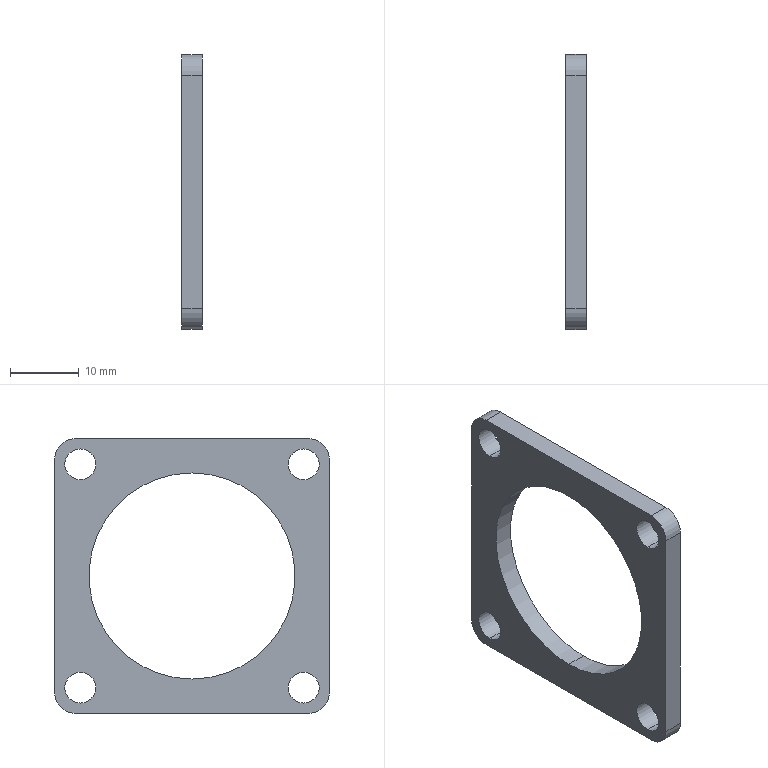Part | SolidWorks | features BaseBody 1 | 1 solid | 20 faces | box 3 x 40 x 40 mm | volume 2465 mm3 | cylinder 14 | plane 6 | commonest cylinder face diameters 4.5 x8 6 x4 30 x2
STEP:
#1=CARTESIAN_POINT('',(298.479,1907.044,-147.5));
#2=VERTEX_POINT('',#1);
#3=CARTESIAN_POINT('',(298.479,1907.044,-177.5));
#4=VERTEX_POINT('',#3);
#5=CARTESIAN_POINT('',(298.479,1907.044,-162.5));
#6=DIRECTION('',(1.,0.,0.));
#7=DIRECTION('',(0.,0.,-1.));
#8=AXIS2_PLACEMENT_3D('',#5,#6,#7);
#9=CIRCLE('',#8,15.);
#10=EDGE_CURVE('',#2,#4,#9,.T.);
#11=ORIENTED_EDGE('',*,*,#10,.F.);
#12=CARTESIAN_POINT('',(301.479,1907.044,-147.5));
#13=VERTEX_POINT('',#12);
#14=CARTESIAN_POINT('',(244.831,1907.044,-147.5));
#15=DIRECTION('',(1.,0.,0.));
#16=VECTOR('',#15,1000.);
#17=LINE('',#14,#16);
#18=EDGE_CURVE('',#2,#13,#17,.T.);
#19=ORIENTED_EDGE('',*,*,#18,.T.);
#20=CARTESIAN_POINT('',(301.479,1907.044,-177.5));
#21=VERTEX_POINT('',#20);
#22=CARTESIAN_POINT('',(301.479,1907.044,-162.5));
#23=DIRECTION('',(-1.,0.,0.));
#24=DIRECTION('',(0.,0.,-1.));
#25=AXIS2_PLACEMENT_3D('',#22,#23,#24);
#26=CIRCLE('',#25,15.);
#27=EDGE_CURVE('',#21,#13,#26,.T.);
#28=ORIENTED_EDGE('',*,*,#27,.F.);
#29=CARTESIAN_POINT('',(244.831,1907.044,-177.5));
#30=DIRECTION('',(1.,0.,0.));
#31=VECTOR('',#30,1000.);
#32=LINE('',#29,#31);
#33=EDGE_CURVE('',#4,#21,#32,.T.);
#34=ORIENTED_EDGE('',*,*,#33,.F.);
#35=EDGE_LOOP('',(#11,#19,#28,#34));
#36=FACE_OUTER_BOUND('',#35,.T.);
#37=CARTESIAN_POINT('',(244.831,1907.044,-162.5));
#38=DIRECTION('',(1.,0.,0.));
#39=DIRECTION('',(0.,0.,-1.));
#40=AXIS2_PLACEMENT_3D('',#37,#38,#39);
#41=CYLINDRICAL_SURFACE('',#40,15.);
#42=ADVANCED_FACE('',(#36),#41,.F.);
#43=CARTESIAN_POINT('',(298.479,1890.781,-176.513));
#44=VERTEX_POINT('',#43);
#45=CARTESIAN_POINT('',(298.479,1890.781,-181.013));
#46=VERTEX_POINT('',#45);
#47=CARTESIAN_POINT('',(298.479,1890.781,-178.763));
#48=DIRECTION('',(1.,0.,0.));
#49=DIRECTION('',(0.,0.,-1.));
#50=AXIS2_PLACEMENT_3D('',#47,#48,#49);
#51=CIRCLE('',#50,2.25);
#52=EDGE_CURVE('',#44,#46,#51,.T.);
#53=ORIENTED_EDGE('',*,*,#52,.F.);
#54=CARTESIAN_POINT('',(301.479,1890.781,-176.513));
#55=VERTEX_POINT('',#54);
#56=CARTESIAN_POINT('',(244.831,1890.781,-176.513));
#57=DIRECTION('',(1.,0.,0.));
#58=VECTOR('',#57,1000.);
#59=LINE('',#56,#58);
#60=EDGE_CURVE('',#44,#55,#59,.T.);
#61=ORIENTED_EDGE('',*,*,#60,.T.);
#62=CARTESIAN_POINT('',(301.479,1890.781,-181.013));
#63=VERTEX_POINT('',#62);
#64=CARTESIAN_POINT('',(301.479,1890.781,-178.763));
#65=DIRECTION('',(-1.,0.,0.));
#66=DIRECTION('',(0.,0.,-1.));
#67=AXIS2_PLACEMENT_3D('',#64,#65,#66);
#68=CIRCLE('',#67,2.25);
#69=EDGE_CURVE('',#63,#55,#68,.T.);
#70=ORIENTED_EDGE('',*,*,#69,.F.);
#71=CARTESIAN_POINT('',(244.831,1890.781,-181.013));
#72=DIRECTION('',(1.,0.,0.));
#73=VECTOR('',#72,1000.);
#74=LINE('',#71,#73);
#75=EDGE_CURVE('',#46,#63,#74,.T.);
#76=ORIENTED_EDGE('',*,*,#75,.F.);
#77=EDGE_LOOP('',(#53,#61,#70,#76));
#78=FACE_OUTER_BOUND('',#77,.T.);
#79=CARTESIAN_POINT('',(244.831,1890.781,-178.763));
#80=DIRECTION('',(1.,0.,0.));
#81=DIRECTION('',(0.,0.,-1.));
#82=AXIS2_PLACEMENT_3D('',#79,#80,#81);
#83=CYLINDRICAL_SURFACE('',#82,2.25);
#84=ADVANCED_FACE('',(#78),#83,.F.);
#85=CARTESIAN_POINT('',(298.479,1890.781,-143.987));
#86=VERTEX_POINT('',#85);
#87=CARTESIAN_POINT('',(298.479,1890.781,-148.487));
#88=VERTEX_POINT('',#87);
#89=CARTESIAN_POINT('',(298.479,1890.781,-146.237));
#90=DIRECTION('',(1.,0.,0.));
#91=DIRECTION('',(0.,0.,-1.));
#92=AXIS2_PLACEMENT_3D('',#89,#90,#91);
#93=CIRCLE('',#92,2.25);
#94=EDGE_CURVE('',#86,#88,#93,.T.);
#95=ORIENTED_EDGE('',*,*,#94,.F.);
#96=CARTESIAN_POINT('',(301.479,1890.781,-143.987));
#97=VERTEX_POINT('',#96);
#98=CARTESIAN_POINT('',(244.831,1890.781,-143.987));
#99=DIRECTION('',(1.,0.,0.));
#100=VECTOR('',#99,1000.);
#101=LINE('',#98,#100);
#102=EDGE_CURVE('',#86,#97,#101,.T.);
#103=ORIENTED_EDGE('',*,*,#102,.T.);
#104=CARTESIAN_POINT('',(301.479,1890.781,-148.487));
#105=VERTEX_POINT('',#104);
#106=CARTESIAN_POINT('',(301.479,1890.781,-146.237));
#107=DIRECTION('',(-1.,0.,0.));
#108=DIRECTION('',(0.,0.,-1.));
#109=AXIS2_PLACEMENT_3D('',#106,#107,#108);
#110=CIRCLE('',#109,2.25);
#111=EDGE_CURVE('',#105,#97,#110,.T.);
#112=ORIENTED_EDGE('',*,*,#111,.F.);
#113=CARTESIAN_POINT('',(244.831,1890.781,-148.487));
#114=DIRECTION('',(1.,0.,0.));
#115=VECTOR('',#114,1000.);
#116=LINE('',#113,#115);
#117=EDGE_CURVE('',#88,#105,#116,.T.);
#118=ORIENTED_EDGE('',*,*,#117,.F.);
#119=EDGE_LOOP('',(#95,#103,#112,#118));
#120=FACE_OUTER_BOUND('',#119,.T.);
#121=CARTESIAN_POINT('',(244.831,1890.781,-146.237));
#122=DIRECTION('',(1.,0.,0.));
#123=DIRECTION('',(0.,0.,-1.));
#124=AXIS2_PLACEMENT_3D('',#121,#122,#123);
#125=CYLINDRICAL_SURFACE('',#124,2.25);
#126=ADVANCED_FACE('',(#120),#125,.F.);
#127=CARTESIAN_POINT('',(298.479,1923.307,-143.987));
#128=VERTEX_POINT('',#127);
#129=CARTESIAN_POINT('',(298.479,1923.307,-148.487));
#130=VERTEX_POINT('',#129);
#131=CARTESIAN_POINT('',(298.479,1923.307,-146.237));
#132=DIRECTION('',(1.,0.,0.));
#133=DIRECTION('',(0.,0.,-1.));
#134=AXIS2_PLACEMENT_3D('',#131,#132,#133);
#135=CIRCLE('',#134,2.25);
#136=EDGE_CURVE('',#128,#130,#135,.T.);
#137=ORIENTED_EDGE('',*,*,#136,.F.);
#138=CARTESIAN_POINT('',(301.479,1923.307,-143.987));
#139=VERTEX_POINT('',#138);
#140=CARTESIAN_POINT('',(244.831,1923.307,-143.987));
#141=DIRECTION('',(1.,0.,0.));
#142=VECTOR('',#141,1000.);
#143=LINE('',#140,#142);
#144=EDGE_CURVE('',#128,#139,#143,.T.);
#145=ORIENTED_EDGE('',*,*,#144,.T.);
#146=CARTESIAN_POINT('',(301.479,1923.307,-148.487));
#147=VERTEX_POINT('',#146);
#148=CARTESIAN_POINT('',(301.479,1923.307,-146.237));
#149=DIRECTION('',(-1.,0.,0.));
#150=DIRECTION('',(0.,0.,-1.));
#151=AXIS2_PLACEMENT_3D('',#148,#149,#150);
#152=CIRCLE('',#151,2.25);
#153=EDGE_CURVE('',#147,#139,#152,.T.);
#154=ORIENTED_EDGE('',*,*,#153,.F.);
#155=CARTESIAN_POINT('',(244.831,1923.307,-148.487));
#156=DIRECTION('',(1.,0.,0.));
#157=VECTOR('',#156,1000.);
#158=LINE('',#155,#157);
#159=EDGE_CURVE('',#130,#147,#158,.T.);
#160=ORIENTED_EDGE('',*,*,#159,.F.);
#161=EDGE_LOOP('',(#137,#145,#154,#160));
#162=FACE_OUTER_BOUND('',#161,.T.);
#163=CARTESIAN_POINT('',(244.831,1923.307,-146.237));
#164=DIRECTION('',(1.,0.,0.));
#165=DIRECTION('',(0.,0.,-1.));
#166=AXIS2_PLACEMENT_3D('',#163,#164,#165);
#167=CYLINDRICAL_SURFACE('',#166,2.25);
#168=ADVANCED_FACE('',(#162),#167,.F.);
#169=CARTESIAN_POINT('',(298.479,1923.307,-176.513));
#170=VERTEX_POINT('',#169);
#171=CARTESIAN_POINT('',(298.479,1923.307,-181.013));
#172=VERTEX_POINT('',#171);
#173=CARTESIAN_POINT('',(298.479,1923.307,-178.763));
#174=DIRECTION('',(1.,0.,0.));
#175=DIRECTION('',(0.,0.,-1.));
#176=AXIS2_PLACEMENT_3D('',#173,#174,#175);
#177=CIRCLE('',#176,2.25);
#178=EDGE_CURVE('',#170,#172,#177,.T.);
#179=ORIENTED_EDGE('',*,*,#178,.F.);
#180=CARTESIAN_POINT('',(301.479,1923.307,-176.513));
#181=VERTEX_POINT('',#180);
#182=CARTESIAN_POINT('',(244.831,1923.307,-176.513));
#183=DIRECTION('',(1.,0.,0.));
#184=VECTOR('',#183,1000.);
#185=LINE('',#182,#184);
#186=EDGE_CURVE('',#170,#181,#185,.T.);
#187=ORIENTED_EDGE('',*,*,#186,.T.);
#188=CARTESIAN_POINT('',(301.479,1923.307,-181.013));
#189=VERTEX_POINT('',#188);
#190=CARTESIAN_POINT('',(301.479,1923.307,-178.763));
#191=DIRECTION('',(-1.,0.,0.));
#192=DIRECTION('',(0.,0.,-1.));
#193=AXIS2_PLACEMENT_3D('',#190,#191,#192);
#194=CIRCLE('',#193,2.25);
#195=EDGE_CURVE('',#189,#181,#194,.T.);
#196=ORIENTED_EDGE('',*,*,#195,.F.);
#197=CARTESIAN_POINT('',(244.831,1923.307,-181.013));
#198=DIRECTION('',(1.,0.,0.));
#199=VECTOR('',#198,1000.);
#200=LINE('',#197,#199);
#201=EDGE_CURVE('',#172,#189,#200,.T.);
#202=ORIENTED_EDGE('',*,*,#201,.F.);
#203=EDGE_LOOP('',(#179,#187,#196,#202));
#204=FACE_OUTER_BOUND('',#203,.T.);
#205=CARTESIAN_POINT('',(244.831,1923.307,-178.763));
#206=DIRECTION('',(1.,0.,0.));
#207=DIRECTION('',(0.,0.,-1.));
#208=AXIS2_PLACEMENT_3D('',#205,#206,#207);
#209=CYLINDRICAL_SURFACE('',#208,2.25);
#210=ADVANCED_FACE('',(#204),#209,.F.);
#211=ORIENTED_EDGE('',*,*,#27,.T.);
#212=CARTESIAN_POINT('',(301.479,1907.044,-162.5));
#213=DIRECTION('',(-1.,0.,0.));
#214=DIRECTION('',(0.,0.,-1.));
#215=AXIS2_PLACEMENT_3D('',#212,#213,#214);
#216=CIRCLE('',#215,15.);
#217=EDGE_CURVE('',#13,#21,#216,.T.);
#218=ORIENTED_EDGE('',*,*,#217,.T.);
#219=EDGE_LOOP('',(#211,#218));
#220=FACE_BOUND('',#219,.T.);
#221=ORIENTED_EDGE('',*,*,#69,.T.);
#222=CARTESIAN_POINT('',(301.479,1890.781,-178.763));
#223=DIRECTION('',(-1.,0.,0.));
#224=DIRECTION('',(0.,0.,-1.));
#225=AXIS2_PLACEMENT_3D('',#222,#223,#224);
#226=CIRCLE('',#225,2.25);
#227=EDGE_CURVE('',#55,#63,#226,.T.);
#228=ORIENTED_EDGE('',*,*,#227,.T.);
#229=EDGE_LOOP('',(#221,#228));
#230=FACE_BOUND('',#229,.T.);
#231=ORIENTED_EDGE('',*,*,#111,.T.);
#232=CARTESIAN_POINT('',(301.479,1890.781,-146.237));
#233=DIRECTION('',(-1.,0.,0.));
#234=DIRECTION('',(0.,0.,-1.));
#235=AXIS2_PLACEMENT_3D('',#232,#233,#234);
#236=CIRCLE('',#235,2.25);
#237=EDGE_CURVE('',#97,#105,#236,.T.);
#238=ORIENTED_EDGE('',*,*,#237,.T.);
#239=EDGE_LOOP('',(#231,#238));
#240=FACE_BOUND('',#239,.T.);
#241=ORIENTED_EDGE('',*,*,#153,.T.);
#242=CARTESIAN_POINT('',(301.479,1923.307,-146.237));
#243=DIRECTION('',(-1.,0.,0.));
#244=DIRECTION('',(0.,0.,-1.));
#245=AXIS2_PLACEMENT_3D('',#242,#243,#244);
#246=CIRCLE('',#245,2.25);
#247=EDGE_CURVE('',#139,#147,#246,.T.);
#248=ORIENTED_EDGE('',*,*,#247,.T.);
#249=EDGE_LOOP('',(#241,#248));
#250=FACE_BOUND('',#249,.T.);
#251=ORIENTED_EDGE('',*,*,#195,.T.);
#252=CARTESIAN_POINT('',(301.479,1923.307,-178.763));
#253=DIRECTION('',(-1.,0.,0.));
#254=DIRECTION('',(0.,0.,-1.));
#255=AXIS2_PLACEMENT_3D('',#252,#253,#254);
#256=CIRCLE('',#255,2.25);
#257=EDGE_CURVE('',#181,#189,#256,.T.);
#258=ORIENTED_EDGE('',*,*,#257,.T.);
#259=EDGE_LOOP('',(#251,#258));
#260=FACE_BOUND('',#259,.T.);
#261=CARTESIAN_POINT('',(301.479,1927.044,-179.5));
#262=VERTEX_POINT('',#261);
#263=CARTESIAN_POINT('',(301.479,1927.044,-145.5));
#264=VERTEX_POINT('',#263);
#265=CARTESIAN_POINT('',(301.479,1927.044,-162.5));
#266=DIRECTION('',(0.,0.,1.));
#267=VECTOR('',#266,1000.);
#268=LINE('',#265,#267);
#269=EDGE_CURVE('',#262,#264,#268,.T.);
#270=ORIENTED_EDGE('',*,*,#269,.T.);
#271=CARTESIAN_POINT('',(301.479,1924.044,-142.5));
#272=VERTEX_POINT('',#271);
#273=CARTESIAN_POINT('',(301.479,1924.044,-145.5));
#274=DIRECTION('',(1.,0.,0.));
#275=DIRECTION('',(0.,0.,-1.));
#276=AXIS2_PLACEMENT_3D('',#273,#274,#275);
#277=CIRCLE('',#276,3.);
#278=EDGE_CURVE('',#264,#272,#277,.T.);
#279=ORIENTED_EDGE('',*,*,#278,.T.);
#280=CARTESIAN_POINT('',(301.479,1890.044,-142.5));
#281=VERTEX_POINT('',#280);
#282=CARTESIAN_POINT('',(301.479,1907.044,-142.5));
#283=DIRECTION('',(0.,-1.,0.));
#284=VECTOR('',#283,1000.);
#285=LINE('',#282,#284);
#286=EDGE_CURVE('',#272,#281,#285,.T.);
#287=ORIENTED_EDGE('',*,*,#286,.T.);
#288=CARTESIAN_POINT('',(301.479,1887.044,-145.5));
#289=VERTEX_POINT('',#288);
#290=CARTESIAN_POINT('',(301.479,1890.044,-145.5));
#291=DIRECTION('',(1.,0.,0.));
#292=DIRECTION('',(0.,0.,-1.));
#293=AXIS2_PLACEMENT_3D('',#290,#291,#292);
#294=CIRCLE('',#293,3.);
#295=EDGE_CURVE('',#281,#289,#294,.T.);
#296=ORIENTED_EDGE('',*,*,#295,.T.);
#297=CARTESIAN_POINT('',(301.479,1887.044,-179.5));
#298=VERTEX_POINT('',#297);
#299=CARTESIAN_POINT('',(301.479,1887.044,-162.5));
#300=DIRECTION('',(0.,0.,-1.));
#301=VECTOR('',#300,1000.);
#302=LINE('',#299,#301);
#303=EDGE_CURVE('',#289,#298,#302,.T.);
#304=ORIENTED_EDGE('',*,*,#303,.T.);
#305=CARTESIAN_POINT('',(301.479,1890.044,-182.5));
#306=VERTEX_POINT('',#305);
#307=CARTESIAN_POINT('',(301.479,1890.044,-179.5));
#308=DIRECTION('',(1.,0.,0.));
#309=DIRECTION('',(0.,0.,-1.));
#310=AXIS2_PLACEMENT_3D('',#307,#308,#309);
#311=CIRCLE('',#310,3.);
#312=EDGE_CURVE('',#298,#306,#311,.T.);
#313=ORIENTED_EDGE('',*,*,#312,.T.);
#314=CARTESIAN_POINT('',(301.479,1924.044,-182.5));
#315=VERTEX_POINT('',#314);
#316=CARTESIAN_POINT('',(301.479,1907.044,-182.5));
#317=DIRECTION('',(0.,1.,0.));
#318=VECTOR('',#317,1000.);
#319=LINE('',#316,#318);
#320=EDGE_CURVE('',#306,#315,#319,.T.);
#321=ORIENTED_EDGE('',*,*,#320,.T.);
#322=CARTESIAN_POINT('',(301.479,1924.044,-179.5));
#323=DIRECTION('',(1.,0.,0.));
#324=DIRECTION('',(0.,0.,-1.));
#325=AXIS2_PLACEMENT_3D('',#322,#323,#324);
#326=CIRCLE('',#325,3.);
#327=EDGE_CURVE('',#315,#262,#326,.T.);
#328=ORIENTED_EDGE('',*,*,#327,.T.);
#329=EDGE_LOOP('',(#270,#279,#287,#296,#304,#313,#321,#328));
#330=FACE_OUTER_BOUND('',#329,.T.);
#331=CARTESIAN_POINT('',(301.479,1907.044,-162.5));
#332=DIRECTION('',(1.,0.,0.));
#333=DIRECTION('',(0.,0.,-1.));
#334=AXIS2_PLACEMENT_3D('',#331,#332,#333);
#335=PLANE('',#334);
#336=ADVANCED_FACE('',(#220,#230,#240,#250,#260,#330),#335,.T.);
#337=ORIENTED_EDGE('',*,*,#18,.F.);
#338=CARTESIAN_POINT('',(298.479,1907.044,-162.5));
#339=DIRECTION('',(1.,0.,0.));
#340=DIRECTION('',(0.,0.,-1.));
#341=AXIS2_PLACEMENT_3D('',#338,#339,#340);
#342=CIRCLE('',#341,15.);
#343=EDGE_CURVE('',#4,#2,#342,.T.);
#344=ORIENTED_EDGE('',*,*,#343,.F.);
#345=ORIENTED_EDGE('',*,*,#33,.T.);
#346=ORIENTED_EDGE('',*,*,#217,.F.);
#347=EDGE_LOOP('',(#337,#344,#345,#346));
#348=FACE_OUTER_BOUND('',#347,.T.);
#349=CARTESIAN_POINT('',(244.831,1907.044,-162.5));
#350=DIRECTION('',(1.,0.,0.));
#351=DIRECTION('',(0.,0.,-1.));
#352=AXIS2_PLACEMENT_3D('',#349,#350,#351);
#353=CYLINDRICAL_SURFACE('',#352,15.);
#354=ADVANCED_FACE('',(#348),#353,.F.);
#355=ORIENTED_EDGE('',*,*,#60,.F.);
#356=CARTESIAN_POINT('',(298.479,1890.781,-178.763));
#357=DIRECTION('',(1.,0.,0.));
#358=DIRECTION('',(0.,0.,-1.));
#359=AXIS2_PLACEMENT_3D('',#356,#357,#358);
#360=CIRCLE('',#359,2.25);
#361=EDGE_CURVE('',#46,#44,#360,.T.);
#362=ORIENTED_EDGE('',*,*,#361,.F.);
#363=ORIENTED_EDGE('',*,*,#75,.T.);
#364=ORIENTED_EDGE('',*,*,#227,.F.);
#365=EDGE_LOOP('',(#355,#362,#363,#364));
#366=FACE_OUTER_BOUND('',#365,.T.);
#367=CARTESIAN_POINT('',(244.831,1890.781,-178.763));
#368=DIRECTION('',(1.,0.,0.));
#369=DIRECTION('',(0.,0.,-1.));
#370=AXIS2_PLACEMENT_3D('',#367,#368,#369);
#371=CYLINDRICAL_SURFACE('',#370,2.25);
#372=ADVANCED_FACE('',(#366),#371,.F.);
#373=ORIENTED_EDGE('',*,*,#102,.F.);
#374=CARTESIAN_POINT('',(298.479,1890.781,-146.237));
#375=DIRECTION('',(1.,0.,0.));
#376=DIRECTION('',(0.,0.,-1.));
#377=AXIS2_PLACEMENT_3D('',#374,#375,#376);
#378=CIRCLE('',#377,2.25);
#379=EDGE_CURVE('',#88,#86,#378,.T.);
#380=ORIENTED_EDGE('',*,*,#379,.F.);
#381=ORIENTED_EDGE('',*,*,#117,.T.);
#382=ORIENTED_EDGE('',*,*,#237,.F.);
#383=EDGE_LOOP('',(#373,#380,#381,#382));
#384=FACE_OUTER_BOUND('',#383,.T.);
#385=CARTESIAN_POINT('',(244.831,1890.781,-146.237));
#386=DIRECTION('',(1.,0.,0.));
#387=DIRECTION('',(0.,0.,-1.));
#388=AXIS2_PLACEMENT_3D('',#385,#386,#387);
#389=CYLINDRICAL_SURFACE('',#388,2.25);
#390=ADVANCED_FACE('',(#384),#389,.F.);
#391=ORIENTED_EDGE('',*,*,#144,.F.);
#392=CARTESIAN_POINT('',(298.479,1923.307,-146.237));
#393=DIRECTION('',(1.,0.,0.));
#394=DIRECTION('',(0.,0.,-1.));
#395=AXIS2_PLACEMENT_3D('',#392,#393,#394);
#396=CIRCLE('',#395,2.25);
#397=EDGE_CURVE('',#130,#128,#396,.T.);
#398=ORIENTED_EDGE('',*,*,#397,.F.);
#399=ORIENTED_EDGE('',*,*,#159,.T.);
#400=ORIENTED_EDGE('',*,*,#247,.F.);
#401=EDGE_LOOP('',(#391,#398,#399,#400));
#402=FACE_OUTER_BOUND('',#401,.T.);
#403=CARTESIAN_POINT('',(244.831,1923.307,-146.237));
#404=DIRECTION('',(1.,0.,0.));
#405=DIRECTION('',(0.,0.,-1.));
#406=AXIS2_PLACEMENT_3D('',#403,#404,#405);
#407=CYLINDRICAL_SURFACE('',#406,2.25);
#408=ADVANCED_FACE('',(#402),#407,.F.);
#409=ORIENTED_EDGE('',*,*,#186,.F.);
#410=CARTESIAN_POINT('',(298.479,1923.307,-178.763));
#411=DIRECTION('',(1.,0.,0.));
#412=DIRECTION('',(0.,0.,-1.));
#413=AXIS2_PLACEMENT_3D('',#410,#411,#412);
#414=CIRCLE('',#413,2.25);
#415=EDGE_CURVE('',#172,#170,#414,.T.);
#416=ORIENTED_EDGE('',*,*,#415,.F.);
#417=ORIENTED_EDGE('',*,*,#201,.T.);
#418=ORIENTED_EDGE('',*,*,#257,.F.);
#419=EDGE_LOOP('',(#409,#416,#417,#418));
#420=FACE_OUTER_BOUND('',#419,.T.);
#421=CARTESIAN_POINT('',(244.831,1923.307,-178.763));
#422=DIRECTION('',(1.,0.,0.));
#423=DIRECTION('',(0.,0.,-1.));
#424=AXIS2_PLACEMENT_3D('',#421,#422,#423);
#425=CYLINDRICAL_SURFACE('',#424,2.25);
#426=ADVANCED_FACE('',(#420),#425,.F.);
#427=CARTESIAN_POINT('',(298.479,1927.044,-145.5));
#428=VERTEX_POINT('',#427);
#429=CARTESIAN_POINT('',(298.479,1927.044,-145.5));
#430=DIRECTION('',(-1.,0.,0.));
#431=VECTOR('',#430,1000.);
#432=LINE('',#429,#431);
#433=EDGE_CURVE('',#264,#428,#432,.T.);
#434=ORIENTED_EDGE('',*,*,#433,.T.);
#435=CARTESIAN_POINT('',(298.479,1924.044,-142.5));
#436=VERTEX_POINT('',#435);
#437=CARTESIAN_POINT('',(298.479,1924.044,-145.5));
#438=DIRECTION('',(1.,0.,0.));
#439=DIRECTION('',(0.,0.,-1.));
#440=AXIS2_PLACEMENT_3D('',#437,#438,#439);
#441=CIRCLE('',#440,3.);
#442=EDGE_CURVE('',#428,#436,#441,.T.);
#443=ORIENTED_EDGE('',*,*,#442,.T.);
#444=CARTESIAN_POINT('',(298.479,1924.044,-142.5));
#445=DIRECTION('',(1.,0.,0.));
#446=VECTOR('',#445,1000.);
#447=LINE('',#444,#446);
#448=EDGE_CURVE('',#436,#272,#447,.T.);
#449=ORIENTED_EDGE('',*,*,#448,.T.);
#450=ORIENTED_EDGE('',*,*,#278,.F.);
#451=EDGE_LOOP('',(#434,#443,#449,#450));
#452=FACE_OUTER_BOUND('',#451,.T.);
#453=CARTESIAN_POINT('',(298.479,1924.044,-145.5));
#454=DIRECTION('',(1.,0.,0.));
#455=DIRECTION('',(0.,0.,-1.));
#456=AXIS2_PLACEMENT_3D('',#453,#454,#455);
#457=CYLINDRICAL_SURFACE('',#456,3.);
#458=ADVANCED_FACE('',(#452),#457,.T.);
#459=ORIENTED_EDGE('',*,*,#269,.F.);
#460=CARTESIAN_POINT('',(298.479,1927.044,-179.5));
#461=VERTEX_POINT('',#460);
#462=CARTESIAN_POINT('',(298.479,1927.044,-179.5));
#463=DIRECTION('',(-1.,0.,0.));
#464=VECTOR('',#463,1000.);
#465=LINE('',#462,#464);
#466=EDGE_CURVE('',#262,#461,#465,.T.);
#467=ORIENTED_EDGE('',*,*,#466,.T.);
#468=CARTESIAN_POINT('',(298.479,1927.044,-142.5));
#469=DIRECTION('',(0.,0.,1.));
#470=VECTOR('',#469,1000.);
#471=LINE('',#468,#470);
#472=EDGE_CURVE('',#461,#428,#471,.T.);
#473=ORIENTED_EDGE('',*,*,#472,.T.);
#474=ORIENTED_EDGE('',*,*,#433,.F.);
#475=EDGE_LOOP('',(#459,#467,#473,#474));
#476=FACE_OUTER_BOUND('',#475,.T.);
#477=CARTESIAN_POINT('',(298.479,1927.044,-142.5));
#478=DIRECTION('',(0.,1.,0.));
#479=DIRECTION('',(0.,0.,1.));
#480=AXIS2_PLACEMENT_3D('',#477,#478,#479);
#481=PLANE('',#480);
#482=ADVANCED_FACE('',(#476),#481,.T.);
#483=CARTESIAN_POINT('',(298.479,1924.044,-182.5));
#484=VERTEX_POINT('',#483);
#485=CARTESIAN_POINT('',(298.479,1924.044,-182.5));
#486=DIRECTION('',(-1.,0.,0.));
#487=VECTOR('',#486,1000.);
#488=LINE('',#485,#487);
#489=EDGE_CURVE('',#315,#484,#488,.T.);
#490=ORIENTED_EDGE('',*,*,#489,.T.);
#491=CARTESIAN_POINT('',(298.479,1924.044,-179.5));
#492=DIRECTION('',(1.,0.,0.));
#493=DIRECTION('',(0.,0.,-1.));
#494=AXIS2_PLACEMENT_3D('',#491,#492,#493);
#495=CIRCLE('',#494,3.);
#496=EDGE_CURVE('',#484,#461,#495,.T.);
#497=ORIENTED_EDGE('',*,*,#496,.T.);
#498=ORIENTED_EDGE('',*,*,#466,.F.);
#499=ORIENTED_EDGE('',*,*,#327,.F.);
#500=EDGE_LOOP('',(#490,#497,#498,#499));
#501=FACE_OUTER_BOUND('',#500,.T.);
#502=CARTESIAN_POINT('',(298.479,1924.044,-179.5));
#503=DIRECTION('',(1.,0.,0.));
#504=DIRECTION('',(0.,0.,-1.));
#505=AXIS2_PLACEMENT_3D('',#502,#503,#504);
#506=CYLINDRICAL_SURFACE('',#505,3.);
#507=ADVANCED_FACE('',(#501),#506,.T.);
#508=CARTESIAN_POINT('',(298.479,1890.044,-182.5));
#509=VERTEX_POINT('',#508);
#510=CARTESIAN_POINT('',(298.479,1927.044,-182.5));
#511=DIRECTION('',(0.,1.,0.));
#512=VECTOR('',#511,1000.);
#513=LINE('',#510,#512);
#514=EDGE_CURVE('',#509,#484,#513,.T.);
#515=ORIENTED_EDGE('',*,*,#514,.T.);
#516=ORIENTED_EDGE('',*,*,#489,.F.);
#517=ORIENTED_EDGE('',*,*,#320,.F.);
#518=CARTESIAN_POINT('',(298.479,1890.044,-182.5));
#519=DIRECTION('',(-1.,0.,0.));
#520=VECTOR('',#519,1000.);
#521=LINE('',#518,#520);
#522=EDGE_CURVE('',#306,#509,#521,.T.);
#523=ORIENTED_EDGE('',*,*,#522,.T.);
#524=EDGE_LOOP('',(#515,#516,#517,#523));
#525=FACE_OUTER_BOUND('',#524,.T.);
#526=CARTESIAN_POINT('',(298.479,1927.044,-182.5));
#527=DIRECTION('',(0.,0.,-1.));
#528=DIRECTION('',(-1.,0.,0.));
#529=AXIS2_PLACEMENT_3D('',#526,#527,#528);
#530=PLANE('',#529);
#531=ADVANCED_FACE('',(#525),#530,.T.);
#532=CARTESIAN_POINT('',(298.479,1887.044,-179.5));
#533=VERTEX_POINT('',#532);
#534=CARTESIAN_POINT('',(298.479,1887.044,-179.5));
#535=DIRECTION('',(-1.,0.,0.));
#536=VECTOR('',#535,1000.);
#537=LINE('',#534,#536);
#538=EDGE_CURVE('',#298,#533,#537,.T.);
#539=ORIENTED_EDGE('',*,*,#538,.T.);
#540=CARTESIAN_POINT('',(298.479,1890.044,-179.5));
#541=DIRECTION('',(1.,0.,0.));
#542=DIRECTION('',(0.,0.,-1.));
#543=AXIS2_PLACEMENT_3D('',#540,#541,#542);
#544=CIRCLE('',#543,3.);
#545=EDGE_CURVE('',#533,#509,#544,.T.);
#546=ORIENTED_EDGE('',*,*,#545,.T.);
#547=ORIENTED_EDGE('',*,*,#522,.F.);
#548=ORIENTED_EDGE('',*,*,#312,.F.);
#549=EDGE_LOOP('',(#539,#546,#547,#548));
#550=FACE_OUTER_BOUND('',#549,.T.);
#551=CARTESIAN_POINT('',(298.479,1890.044,-179.5));
#552=DIRECTION('',(1.,0.,0.));
#553=DIRECTION('',(0.,0.,-1.));
#554=AXIS2_PLACEMENT_3D('',#551,#552,#553);
#555=CYLINDRICAL_SURFACE('',#554,3.);
#556=ADVANCED_FACE('',(#550),#555,.T.);
#557=CARTESIAN_POINT('',(298.479,1887.044,-145.5));
#558=VERTEX_POINT('',#557);
#559=CARTESIAN_POINT('',(298.479,1887.044,-182.5));
#560=DIRECTION('',(0.,0.,-1.));
#561=VECTOR('',#560,1000.);
#562=LINE('',#559,#561);
#563=EDGE_CURVE('',#558,#533,#562,.T.);
#564=ORIENTED_EDGE('',*,*,#563,.T.);
#565=ORIENTED_EDGE('',*,*,#538,.F.);
#566=ORIENTED_EDGE('',*,*,#303,.F.);
#567=CARTESIAN_POINT('',(298.479,1887.044,-145.5));
#568=DIRECTION('',(-1.,0.,0.));
#569=VECTOR('',#568,1000.);
#570=LINE('',#567,#569);
#571=EDGE_CURVE('',#289,#558,#570,.T.);
#572=ORIENTED_EDGE('',*,*,#571,.T.);
#573=EDGE_LOOP('',(#564,#565,#566,#572));
#574=FACE_OUTER_BOUND('',#573,.T.);
#575=CARTESIAN_POINT('',(298.479,1887.044,-182.5));
#576=DIRECTION('',(0.,-1.,0.));
#577=DIRECTION('',(0.,0.,-1.));
#578=AXIS2_PLACEMENT_3D('',#575,#576,#577);
#579=PLANE('',#578);
#580=ADVANCED_FACE('',(#574),#579,.T.);
#581=CARTESIAN_POINT('',(298.479,1890.044,-142.5));
#582=VERTEX_POINT('',#581);
#583=CARTESIAN_POINT('',(298.479,1890.044,-142.5));
#584=DIRECTION('',(-1.,0.,0.));
#585=VECTOR('',#584,1000.);
#586=LINE('',#583,#585);
#587=EDGE_CURVE('',#281,#582,#586,.T.);
#588=ORIENTED_EDGE('',*,*,#587,.T.);
#589=CARTESIAN_POINT('',(298.479,1890.044,-145.5));
#590=DIRECTION('',(1.,0.,0.));
#591=DIRECTION('',(0.,0.,-1.));
#592=AXIS2_PLACEMENT_3D('',#589,#590,#591);
#593=CIRCLE('',#592,3.);
#594=EDGE_CURVE('',#582,#558,#593,.T.);
#595=ORIENTED_EDGE('',*,*,#594,.T.);
#596=ORIENTED_EDGE('',*,*,#571,.F.);
#597=ORIENTED_EDGE('',*,*,#295,.F.);
#598=EDGE_LOOP('',(#588,#595,#596,#597));
#599=FACE_OUTER_BOUND('',#598,.T.);
#600=CARTESIAN_POINT('',(298.479,1890.044,-145.5));
#601=DIRECTION('',(1.,0.,0.));
#602=DIRECTION('',(0.,0.,-1.));
#603=AXIS2_PLACEMENT_3D('',#600,#601,#602);
#604=CYLINDRICAL_SURFACE('',#603,3.);
#605=ADVANCED_FACE('',(#599),#604,.T.);
#606=ORIENTED_EDGE('',*,*,#286,.F.);
#607=ORIENTED_EDGE('',*,*,#448,.F.);
#608=CARTESIAN_POINT('',(298.479,1887.044,-142.5));
#609=DIRECTION('',(0.,-1.,0.));
#610=VECTOR('',#609,1000.);
#611=LINE('',#608,#610);
#612=EDGE_CURVE('',#436,#582,#611,.T.);
#613=ORIENTED_EDGE('',*,*,#612,.T.);
#614=ORIENTED_EDGE('',*,*,#587,.F.);
#615=EDGE_LOOP('',(#606,#607,#613,#614));
#616=FACE_OUTER_BOUND('',#615,.T.);
#617=CARTESIAN_POINT('',(298.479,1887.044,-142.5));
#618=DIRECTION('',(0.,0.,1.));
#619=DIRECTION('',(1.,0.,0.));
#620=AXIS2_PLACEMENT_3D('',#617,#618,#619);
#621=PLANE('',#620);
#622=ADVANCED_FACE('',(#616),#621,.T.);
#623=ORIENTED_EDGE('',*,*,#343,.T.);
#624=ORIENTED_EDGE('',*,*,#10,.T.);
#625=EDGE_LOOP('',(#623,#624));
#626=FACE_BOUND('',#625,.T.);
#627=ORIENTED_EDGE('',*,*,#361,.T.);
#628=ORIENTED_EDGE('',*,*,#52,.T.);
#629=EDGE_LOOP('',(#627,#628));
#630=FACE_BOUND('',#629,.T.);
#631=ORIENTED_EDGE('',*,*,#379,.T.);
#632=ORIENTED_EDGE('',*,*,#94,.T.);
#633=EDGE_LOOP('',(#631,#632));
#634=FACE_BOUND('',#633,.T.);
#635=ORIENTED_EDGE('',*,*,#397,.T.);
#636=ORIENTED_EDGE('',*,*,#136,.T.);
#637=EDGE_LOOP('',(#635,#636));
#638=FACE_BOUND('',#637,.T.);
#639=ORIENTED_EDGE('',*,*,#415,.T.);
#640=ORIENTED_EDGE('',*,*,#178,.T.);
#641=EDGE_LOOP('',(#639,#640));
#642=FACE_BOUND('',#641,.T.);
#643=ORIENTED_EDGE('',*,*,#472,.F.);
#644=ORIENTED_EDGE('',*,*,#496,.F.);
#645=ORIENTED_EDGE('',*,*,#514,.F.);
#646=ORIENTED_EDGE('',*,*,#545,.F.);
#647=ORIENTED_EDGE('',*,*,#563,.F.);
#648=ORIENTED_EDGE('',*,*,#594,.F.);
#649=ORIENTED_EDGE('',*,*,#612,.F.);
#650=ORIENTED_EDGE('',*,*,#442,.F.);
#651=EDGE_LOOP('',(#643,#644,#645,#646,#647,#648,#649,#650));
#652=FACE_OUTER_BOUND('',#651,.T.);
#653=CARTESIAN_POINT('',(298.479,1907.044,-162.5));
#654=DIRECTION('',(1.,0.,0.));
#655=DIRECTION('',(0.,0.,-1.));
#656=AXIS2_PLACEMENT_3D('',#653,#654,#655);
#657=PLANE('',#656);
#658=ADVANCED_FACE('',(#626,#630,#634,#638,#642,#652),#657,.F.);
#659=CLOSED_SHELL('',(#42,#84,#126,#168,#210,#336,#354,#372,#390,#408,#426,#458,#482,#507,#531,#556,#580,#605,#622,#658));
#660=MANIFOLD_SOLID_BREP('',#659);
#661=CARTESIAN_POINT('',(0.,0.,0.));
#662=DIRECTION('',(0.,0.,1.));
#663=DIRECTION('',(1.,0.,0.));
#664=AXIS2_PLACEMENT_3D('',#661,#662,#663);
#665=(LENGTH_UNIT()NAMED_UNIT(*)SI_UNIT(.MILLI.,.METRE.));
#666=UNCERTAINTY_MEASURE_WITH_UNIT(LENGTH_MEASURE(0.00001),#665,'','');
#667=(NAMED_UNIT(*)PLANE_ANGLE_UNIT()SI_UNIT($,.RADIAN.));
#668=(NAMED_UNIT(*)SI_UNIT($,.STERADIAN.)SOLID_ANGLE_UNIT());
#669=(GEOMETRIC_REPRESENTATION_CONTEXT(3)GLOBAL_UNCERTAINTY_ASSIGNED_CONTEXT((#666))GLOBAL_UNIT_ASSIGNED_CONTEXT((#665,#667,#668))REPRESENTATION_CONTEXT('',''));
#670=ADVANCED_BREP_SHAPE_REPRESENTATION('',(#660,#664),#669);